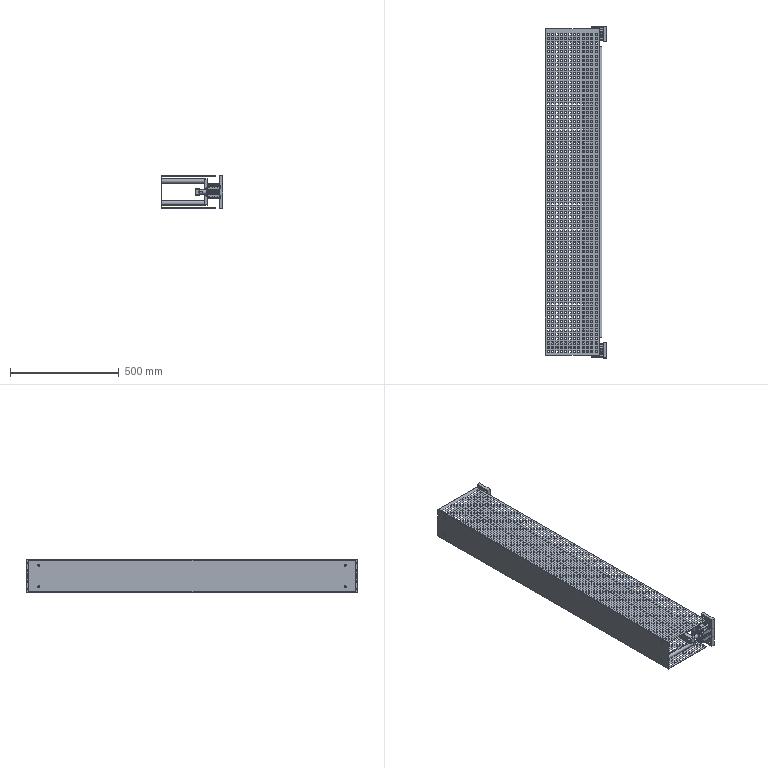Part | SolidWorks | 16 solids | 7952 faces | volume 4434874 mm3 | plane 7405 | cylinder 375 | cone 168 | spline 4 | commonest cylinder face diameters 0.4 x92 11 x44 9 x40 6.647 x32 20 x22 0.8 x20